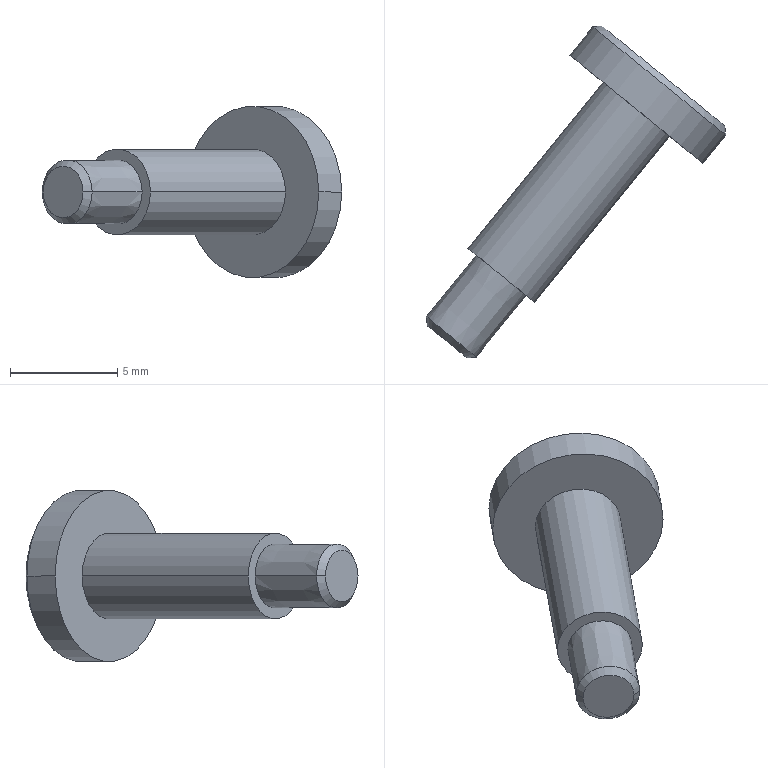Part | SolidWorks | features BaseBody 1 | 1 solid | 14 faces | box 13.983 x 15.505 x 8 mm | volume 252.958 mm3 | cone 6 | cylinder 4 | plane 4 | commonest cylinder face diameters 4 x2 8 x2
STEP:
#1=CARTESIAN_POINT('',(550.561,-174.02,330.545));
#2=VERTEX_POINT('',#1);
#3=CARTESIAN_POINT('',(553.665,-176.544,330.545));
#4=VERTEX_POINT('',#3);
#5=CARTESIAN_POINT('',(552.113,-175.282,330.545));
#6=DIRECTION('',(0.6309,0.7758,-0.000000012));
#7=DIRECTION('',(-0.7758,0.6309,0.));
#8=AXIS2_PLACEMENT_3D('',#5,#6,#7);
#9=CIRCLE('',#8,2.);
#10=EDGE_CURVE('',#2,#4,#9,.T.);
#11=ORIENTED_EDGE('',*,*,#10,.T.);
#12=CARTESIAN_POINT('',(559.974,-168.786,330.545));
#13=VERTEX_POINT('',#12);
#14=CARTESIAN_POINT('',(559.974,-168.786,330.545));
#15=DIRECTION('',(0.6309,0.7758,-0.000000012));
#16=VECTOR('',#15,1000.);
#17=LINE('',#14,#16);
#18=EDGE_CURVE('',#4,#13,#17,.T.);
#19=ORIENTED_EDGE('',*,*,#18,.T.);
#20=CARTESIAN_POINT('',(556.871,-166.262,330.545));
#21=VERTEX_POINT('',#20);
#22=CARTESIAN_POINT('',(558.422,-167.524,330.545));
#23=DIRECTION('',(-0.6309,-0.7758,0.000000012));
#24=DIRECTION('',(-0.7758,0.6309,0.));
#25=AXIS2_PLACEMENT_3D('',#22,#23,#24);
#26=CIRCLE('',#25,2.);
#27=EDGE_CURVE('',#13,#21,#26,.T.);
#28=ORIENTED_EDGE('',*,*,#27,.T.);
#29=CARTESIAN_POINT('',(556.871,-166.262,330.545));
#30=DIRECTION('',(0.6309,0.7758,-0.000000012));
#31=VECTOR('',#30,1000.);
#32=LINE('',#29,#31);
#33=EDGE_CURVE('',#2,#21,#32,.T.);
#34=ORIENTED_EDGE('',*,*,#33,.F.);
#35=EDGE_LOOP('',(#11,#19,#28,#34));
#36=FACE_OUTER_BOUND('',#35,.T.);
#37=CARTESIAN_POINT('',(558.422,-167.524,330.545));
#38=DIRECTION('',(0.6309,0.7758,-0.000000012));
#39=DIRECTION('',(-0.7758,0.6309,0.));
#40=AXIS2_PLACEMENT_3D('',#37,#38,#39);
#41=CYLINDRICAL_SURFACE('',#40,2.);
#42=ADVANCED_FACE('',(#36),#41,.T.);
#43=CARTESIAN_POINT('',(561.526,-170.047,330.545));
#44=VERTEX_POINT('',#43);
#45=CARTESIAN_POINT('',(555.319,-165.,330.545));
#46=VERTEX_POINT('',#45);
#47=CARTESIAN_POINT('',(558.422,-167.524,330.545));
#48=DIRECTION('',(-0.6309,-0.7758,0.000000012));
#49=DIRECTION('',(-0.7758,0.6309,0.));
#50=AXIS2_PLACEMENT_3D('',#47,#48,#49);
#51=CIRCLE('',#50,4.);
#52=EDGE_CURVE('',#44,#46,#51,.T.);
#53=ORIENTED_EDGE('',*,*,#52,.F.);
#54=CARTESIAN_POINT('',(562.598,-168.728,330.545));
#55=VERTEX_POINT('',#54);
#56=CARTESIAN_POINT('',(562.788,-168.496,330.545));
#57=DIRECTION('',(0.6309,0.7758,-0.000000012));
#58=VECTOR('',#57,1000.);
#59=LINE('',#56,#58);
#60=EDGE_CURVE('',#44,#55,#59,.T.);
#61=ORIENTED_EDGE('',*,*,#60,.T.);
#62=CARTESIAN_POINT('',(556.392,-163.681,330.545));
#63=VERTEX_POINT('',#62);
#64=CARTESIAN_POINT('',(559.495,-166.205,330.545));
#65=DIRECTION('',(-0.6309,-0.7758,0.000000012));
#66=DIRECTION('',(-0.7758,0.6309,0.));
#67=AXIS2_PLACEMENT_3D('',#64,#65,#66);
#68=CIRCLE('',#67,4.);
#69=EDGE_CURVE('',#55,#63,#68,.T.);
#70=ORIENTED_EDGE('',*,*,#69,.T.);
#71=CARTESIAN_POINT('',(556.581,-163.448,330.545));
#72=DIRECTION('',(0.6309,0.7758,-0.000000012));
#73=VECTOR('',#72,1000.);
#74=LINE('',#71,#73);
#75=EDGE_CURVE('',#46,#63,#74,.T.);
#76=ORIENTED_EDGE('',*,*,#75,.F.);
#77=EDGE_LOOP('',(#53,#61,#70,#76));
#78=FACE_OUTER_BOUND('',#77,.T.);
#79=CARTESIAN_POINT('',(559.684,-165.972,330.545));
#80=DIRECTION('',(0.6309,0.7758,-0.000000012));
#81=DIRECTION('',(-0.7758,0.6309,0.));
#82=AXIS2_PLACEMENT_3D('',#79,#80,#81);
#83=CYLINDRICAL_SURFACE('',#82,4.);
#84=ADVANCED_FACE('',(#78),#83,.T.);
#85=CARTESIAN_POINT('',(548.615,-177.207,330.545));
#86=VERTEX_POINT('',#85);
#87=CARTESIAN_POINT('',(550.942,-179.099,330.545));
#88=VERTEX_POINT('',#87);
#89=CARTESIAN_POINT('',(549.779,-178.153,330.545));
#90=DIRECTION('',(0.6309,0.7758,-0.000000012));
#91=DIRECTION('',(-0.000000031,0.00000001,-1.));
#92=AXIS2_PLACEMENT_3D('',#89,#90,#91);
#93=CIRCLE('',#92,1.499);
#94=EDGE_CURVE('',#86,#88,#93,.T.);
#95=ORIENTED_EDGE('',*,*,#94,.T.);
#96=CARTESIAN_POINT('',(553.277,-176.228,330.545));
#97=VERTEX_POINT('',#96);
#98=CARTESIAN_POINT('',(553.277,-176.228,330.545));
#99=DIRECTION('',(0.6311,0.7757,-0.000000012));
#100=VECTOR('',#99,1000.);
#101=LINE('',#98,#100);
#102=EDGE_CURVE('',#88,#97,#101,.T.);
#103=ORIENTED_EDGE('',*,*,#102,.T.);
#104=CARTESIAN_POINT('',(550.949,-174.336,330.545));
#105=VERTEX_POINT('',#104);
#106=CARTESIAN_POINT('',(552.113,-175.282,330.545));
#107=DIRECTION('',(0.6309,0.7758,-0.000000012));
#108=DIRECTION('',(-0.7758,0.6309,0.));
#109=AXIS2_PLACEMENT_3D('',#106,#107,#108);
#110=CIRCLE('',#109,1.5);
#111=EDGE_CURVE('',#105,#97,#110,.T.);
#112=ORIENTED_EDGE('',*,*,#111,.F.);
#113=CARTESIAN_POINT('',(550.949,-174.336,330.545));
#114=DIRECTION('',(0.6308,0.7759,-0.000000012));
#115=VECTOR('',#114,1000.);
#116=LINE('',#113,#115);
#117=EDGE_CURVE('',#86,#105,#116,.T.);
#118=ORIENTED_EDGE('',*,*,#117,.F.);
#119=EDGE_LOOP('',(#95,#103,#112,#118));
#120=FACE_OUTER_BOUND('',#119,.T.);
#121=CARTESIAN_POINT('',(552.113,-175.282,330.545));
#122=DIRECTION('',(0.6309,0.7758,-0.000000012));
#123=DIRECTION('',(-0.7758,0.6309,0.));
#124=AXIS2_PLACEMENT_3D('',#121,#122,#123);
#125=CONICAL_SURFACE('',#124,1.5,0.0001745);
#126=ADVANCED_FACE('',(#120),#125,.T.);
#127=CARTESIAN_POINT('',(562.555,-168.306,330.545));
#128=VERTEX_POINT('',#127);
#129=CARTESIAN_POINT('',(556.814,-163.638,330.545));
#130=VERTEX_POINT('',#129);
#131=CARTESIAN_POINT('',(559.684,-165.972,330.545));
#132=DIRECTION('',(-0.6309,-0.7758,0.000000012));
#133=DIRECTION('',(0.7758,-0.6309,0.));
#134=AXIS2_PLACEMENT_3D('',#131,#132,#133);
#135=CIRCLE('',#134,3.7);
#136=EDGE_CURVE('',#128,#130,#135,.T.);
#137=ORIENTED_EDGE('',*,*,#136,.T.);
#138=CARTESIAN_POINT('',(556.392,-163.681,330.545));
#139=DIRECTION('',(-0.9947,-0.1025,0.000000009));
#140=VECTOR('',#139,1000.);
#141=LINE('',#138,#140);
#142=EDGE_CURVE('',#130,#63,#141,.T.);
#143=ORIENTED_EDGE('',*,*,#142,.T.);
#144=ORIENTED_EDGE('',*,*,#69,.F.);
#145=CARTESIAN_POINT('',(562.598,-168.728,330.545));
#146=DIRECTION('',(0.1025,-0.9947,0.000000009));
#147=VECTOR('',#146,1000.);
#148=LINE('',#145,#147);
#149=EDGE_CURVE('',#128,#55,#148,.T.);
#150=ORIENTED_EDGE('',*,*,#149,.F.);
#151=EDGE_LOOP('',(#137,#143,#144,#150));
#152=FACE_OUTER_BOUND('',#151,.T.);
#153=CARTESIAN_POINT('',(559.495,-166.205,330.545));
#154=DIRECTION('',(-0.6309,-0.7758,0.000000012));
#155=DIRECTION('',(0.7758,-0.6309,0.));
#156=AXIS2_PLACEMENT_3D('',#153,#154,#155);
#157=CONICAL_SURFACE('',#156,4.,0.7854);
#158=ADVANCED_FACE('',(#152),#157,.T.);
#159=CARTESIAN_POINT('',(548.659,-177.629,330.545));
#160=VERTEX_POINT('',#159);
#161=CARTESIAN_POINT('',(550.52,-179.142,330.545));
#162=VERTEX_POINT('',#161);
#163=CARTESIAN_POINT('',(549.589,-178.385,330.545));
#164=DIRECTION('',(0.6309,0.7758,-0.000000012));
#165=DIRECTION('',(-0.7758,0.6309,0.));
#166=AXIS2_PLACEMENT_3D('',#163,#164,#165);
#167=CIRCLE('',#166,1.199);
#168=EDGE_CURVE('',#160,#162,#167,.T.);
#169=ORIENTED_EDGE('',*,*,#168,.T.);
#170=CARTESIAN_POINT('',(550.942,-179.099,330.545));
#171=DIRECTION('',(0.9947,0.1024,-0.000000009));
#172=VECTOR('',#171,1000.);
#173=LINE('',#170,#172);
#174=EDGE_CURVE('',#162,#88,#173,.T.);
#175=ORIENTED_EDGE('',*,*,#174,.T.);
#176=ORIENTED_EDGE('',*,*,#94,.F.);
#177=CARTESIAN_POINT('',(548.615,-177.207,330.545));
#178=DIRECTION('',(-0.1026,0.9947,-0.000000009));
#179=VECTOR('',#178,1000.);
#180=LINE('',#177,#179);
#181=EDGE_CURVE('',#160,#86,#180,.T.);
#182=ORIENTED_EDGE('',*,*,#181,.F.);
#183=EDGE_LOOP('',(#169,#175,#176,#182));
#184=FACE_OUTER_BOUND('',#183,.T.);
#185=CARTESIAN_POINT('',(549.779,-178.153,330.545));
#186=DIRECTION('',(0.6309,0.7758,-0.000000012));
#187=DIRECTION('',(-0.7758,0.6309,0.));
#188=AXIS2_PLACEMENT_3D('',#185,#186,#187);
#189=CONICAL_SURFACE('',#188,1.499,0.7855);
#190=ADVANCED_FACE('',(#184),#189,.T.);
#191=ORIENTED_EDGE('',*,*,#18,.F.);
#192=CARTESIAN_POINT('',(552.113,-175.282,330.545));
#193=DIRECTION('',(0.6309,0.7758,-0.000000012));
#194=DIRECTION('',(-0.7758,0.6309,0.));
#195=AXIS2_PLACEMENT_3D('',#192,#193,#194);
#196=CIRCLE('',#195,2.);
#197=EDGE_CURVE('',#4,#2,#196,.T.);
#198=ORIENTED_EDGE('',*,*,#197,.T.);
#199=ORIENTED_EDGE('',*,*,#33,.T.);
#200=CARTESIAN_POINT('',(558.422,-167.524,330.545));
#201=DIRECTION('',(-0.6309,-0.7758,0.000000012));
#202=DIRECTION('',(-0.7758,0.6309,0.));
#203=AXIS2_PLACEMENT_3D('',#200,#201,#202);
#204=CIRCLE('',#203,2.);
#205=EDGE_CURVE('',#21,#13,#204,.T.);
#206=ORIENTED_EDGE('',*,*,#205,.T.);
#207=EDGE_LOOP('',(#191,#198,#199,#206));
#208=FACE_OUTER_BOUND('',#207,.T.);
#209=CARTESIAN_POINT('',(558.422,-167.524,330.545));
#210=DIRECTION('',(0.6309,0.7758,-0.000000012));
#211=DIRECTION('',(-0.7758,0.6309,0.));
#212=AXIS2_PLACEMENT_3D('',#209,#210,#211);
#213=CYLINDRICAL_SURFACE('',#212,2.);
#214=ADVANCED_FACE('',(#208),#213,.T.);
#215=CARTESIAN_POINT('',(558.422,-167.524,330.545));
#216=DIRECTION('',(-0.6309,-0.7758,0.000000012));
#217=DIRECTION('',(-0.7758,0.6309,0.));
#218=AXIS2_PLACEMENT_3D('',#215,#216,#217);
#219=CIRCLE('',#218,4.);
#220=EDGE_CURVE('',#46,#44,#219,.T.);
#221=ORIENTED_EDGE('',*,*,#220,.T.);
#222=ORIENTED_EDGE('',*,*,#52,.T.);
#223=EDGE_LOOP('',(#221,#222));
#224=FACE_OUTER_BOUND('',#223,.T.);
#225=ORIENTED_EDGE('',*,*,#205,.F.);
#226=ORIENTED_EDGE('',*,*,#27,.F.);
#227=EDGE_LOOP('',(#225,#226));
#228=FACE_BOUND('',#227,.T.);
#229=CARTESIAN_POINT('',(558.422,-167.524,330.545));
#230=DIRECTION('',(-0.6309,-0.7758,0.000000012));
#231=DIRECTION('',(0.7758,-0.6309,0.));
#232=AXIS2_PLACEMENT_3D('',#229,#230,#231);
#233=PLANE('',#232);
#234=ADVANCED_FACE('',(#224,#228),#233,.T.);
#235=ORIENTED_EDGE('',*,*,#10,.F.);
#236=ORIENTED_EDGE('',*,*,#197,.F.);
#237=EDGE_LOOP('',(#235,#236));
#238=FACE_OUTER_BOUND('',#237,.T.);
#239=ORIENTED_EDGE('',*,*,#111,.T.);
#240=CARTESIAN_POINT('',(552.113,-175.282,330.545));
#241=DIRECTION('',(0.6309,0.7758,-0.000000012));
#242=DIRECTION('',(-0.7758,0.6309,0.));
#243=AXIS2_PLACEMENT_3D('',#240,#241,#242);
#244=CIRCLE('',#243,1.5);
#245=EDGE_CURVE('',#97,#105,#244,.T.);
#246=ORIENTED_EDGE('',*,*,#245,.T.);
#247=EDGE_LOOP('',(#239,#246));
#248=FACE_BOUND('',#247,.T.);
#249=CARTESIAN_POINT('',(552.113,-175.282,330.545));
#250=DIRECTION('',(-0.6309,-0.7758,0.000000012));
#251=DIRECTION('',(0.7758,-0.6309,0.));
#252=AXIS2_PLACEMENT_3D('',#249,#250,#251);
#253=PLANE('',#252);
#254=ADVANCED_FACE('',(#238,#248),#253,.T.);
#255=ORIENTED_EDGE('',*,*,#60,.F.);
#256=ORIENTED_EDGE('',*,*,#220,.F.);
#257=ORIENTED_EDGE('',*,*,#75,.T.);
#258=CARTESIAN_POINT('',(559.495,-166.205,330.545));
#259=DIRECTION('',(-0.6309,-0.7758,0.000000012));
#260=DIRECTION('',(-0.7758,0.6309,0.));
#261=AXIS2_PLACEMENT_3D('',#258,#259,#260);
#262=CIRCLE('',#261,4.);
#263=EDGE_CURVE('',#63,#55,#262,.T.);
#264=ORIENTED_EDGE('',*,*,#263,.T.);
#265=EDGE_LOOP('',(#255,#256,#257,#264));
#266=FACE_OUTER_BOUND('',#265,.T.);
#267=CARTESIAN_POINT('',(559.684,-165.972,330.545));
#268=DIRECTION('',(0.6309,0.7758,-0.000000012));
#269=DIRECTION('',(-0.7758,0.6309,0.));
#270=AXIS2_PLACEMENT_3D('',#267,#268,#269);
#271=CYLINDRICAL_SURFACE('',#270,4.);
#272=ADVANCED_FACE('',(#266),#271,.T.);
#273=ORIENTED_EDGE('',*,*,#102,.F.);
#274=CARTESIAN_POINT('',(549.779,-178.153,330.545));
#275=DIRECTION('',(0.6309,0.7758,-0.000000012));
#276=DIRECTION('',(-0.000000031,0.00000001,-1.));
#277=AXIS2_PLACEMENT_3D('',#274,#275,#276);
#278=CIRCLE('',#277,1.499);
#279=EDGE_CURVE('',#88,#86,#278,.T.);
#280=ORIENTED_EDGE('',*,*,#279,.T.);
#281=ORIENTED_EDGE('',*,*,#117,.T.);
#282=ORIENTED_EDGE('',*,*,#245,.F.);
#283=EDGE_LOOP('',(#273,#280,#281,#282));
#284=FACE_OUTER_BOUND('',#283,.T.);
#285=CARTESIAN_POINT('',(552.113,-175.282,330.545));
#286=DIRECTION('',(0.6309,0.7758,-0.000000012));
#287=DIRECTION('',(-0.7758,0.6309,0.));
#288=AXIS2_PLACEMENT_3D('',#285,#286,#287);
#289=CONICAL_SURFACE('',#288,1.5,0.0001745);
#290=ADVANCED_FACE('',(#284),#289,.T.);
#291=ORIENTED_EDGE('',*,*,#142,.F.);
#292=CARTESIAN_POINT('',(559.684,-165.972,330.545));
#293=DIRECTION('',(-0.6309,-0.7758,0.000000012));
#294=DIRECTION('',(0.7758,-0.6309,0.));
#295=AXIS2_PLACEMENT_3D('',#292,#293,#294);
#296=CIRCLE('',#295,3.7);
#297=EDGE_CURVE('',#130,#128,#296,.T.);
#298=ORIENTED_EDGE('',*,*,#297,.T.);
#299=ORIENTED_EDGE('',*,*,#149,.T.);
#300=ORIENTED_EDGE('',*,*,#263,.F.);
#301=EDGE_LOOP('',(#291,#298,#299,#300));
#302=FACE_OUTER_BOUND('',#301,.T.);
#303=CARTESIAN_POINT('',(559.495,-166.205,330.545));
#304=DIRECTION('',(-0.6309,-0.7758,0.000000012));
#305=DIRECTION('',(0.7758,-0.6309,0.));
#306=AXIS2_PLACEMENT_3D('',#303,#304,#305);
#307=CONICAL_SURFACE('',#306,4.,0.7854);
#308=ADVANCED_FACE('',(#302),#307,.T.);
#309=ORIENTED_EDGE('',*,*,#174,.F.);
#310=CARTESIAN_POINT('',(549.589,-178.385,330.545));
#311=DIRECTION('',(0.6309,0.7758,-0.000000012));
#312=DIRECTION('',(-0.7758,0.6309,0.));
#313=AXIS2_PLACEMENT_3D('',#310,#311,#312);
#314=CIRCLE('',#313,1.199);
#315=EDGE_CURVE('',#162,#160,#314,.T.);
#316=ORIENTED_EDGE('',*,*,#315,.T.);
#317=ORIENTED_EDGE('',*,*,#181,.T.);
#318=ORIENTED_EDGE('',*,*,#279,.F.);
#319=EDGE_LOOP('',(#309,#316,#317,#318));
#320=FACE_OUTER_BOUND('',#319,.T.);
#321=CARTESIAN_POINT('',(549.779,-178.153,330.545));
#322=DIRECTION('',(0.6309,0.7758,-0.000000012));
#323=DIRECTION('',(-0.7758,0.6309,0.));
#324=AXIS2_PLACEMENT_3D('',#321,#322,#323);
#325=CONICAL_SURFACE('',#324,1.499,0.7855);
#326=ADVANCED_FACE('',(#320),#325,.T.);
#327=ORIENTED_EDGE('',*,*,#136,.F.);
#328=ORIENTED_EDGE('',*,*,#297,.F.);
#329=EDGE_LOOP('',(#327,#328));
#330=FACE_OUTER_BOUND('',#329,.T.);
#331=CARTESIAN_POINT('',(559.684,-165.972,330.545));
#332=DIRECTION('',(-0.6309,-0.7758,0.000000012));
#333=DIRECTION('',(0.7758,-0.6309,0.));
#334=AXIS2_PLACEMENT_3D('',#331,#332,#333);
#335=PLANE('',#334);
#336=ADVANCED_FACE('',(#330),#335,.F.);
#337=ORIENTED_EDGE('',*,*,#168,.F.);
#338=ORIENTED_EDGE('',*,*,#315,.F.);
#339=EDGE_LOOP('',(#337,#338));
#340=FACE_OUTER_BOUND('',#339,.T.);
#341=CARTESIAN_POINT('',(549.589,-178.385,330.545));
#342=DIRECTION('',(-0.6309,-0.7758,0.000000012));
#343=DIRECTION('',(0.7758,-0.6309,0.));
#344=AXIS2_PLACEMENT_3D('',#341,#342,#343);
#345=PLANE('',#344);
#346=ADVANCED_FACE('',(#340),#345,.T.);
#347=CLOSED_SHELL('',(#42,#84,#126,#158,#190,#214,#234,#254,#272,#290,#308,#326,#336,#346));
#348=MANIFOLD_SOLID_BREP('',#347);
#349=CARTESIAN_POINT('',(0.,0.,0.));
#350=DIRECTION('',(0.,0.,1.));
#351=DIRECTION('',(1.,0.,0.));
#352=AXIS2_PLACEMENT_3D('',#349,#350,#351);
#353=(LENGTH_UNIT()NAMED_UNIT(*)SI_UNIT(.MILLI.,.METRE.));
#354=UNCERTAINTY_MEASURE_WITH_UNIT(LENGTH_MEASURE(0.00001),#353,'','');
#355=(NAMED_UNIT(*)PLANE_ANGLE_UNIT()SI_UNIT($,.RADIAN.));
#356=(NAMED_UNIT(*)SI_UNIT($,.STERADIAN.)SOLID_ANGLE_UNIT());
#357=(GEOMETRIC_REPRESENTATION_CONTEXT(3)GLOBAL_UNCERTAINTY_ASSIGNED_CONTEXT((#354))GLOBAL_UNIT_ASSIGNED_CONTEXT((#353,#355,#356))REPRESENTATION_CONTEXT('',''));
#358=ADVANCED_BREP_SHAPE_REPRESENTATION('',(#348,#352),#357);